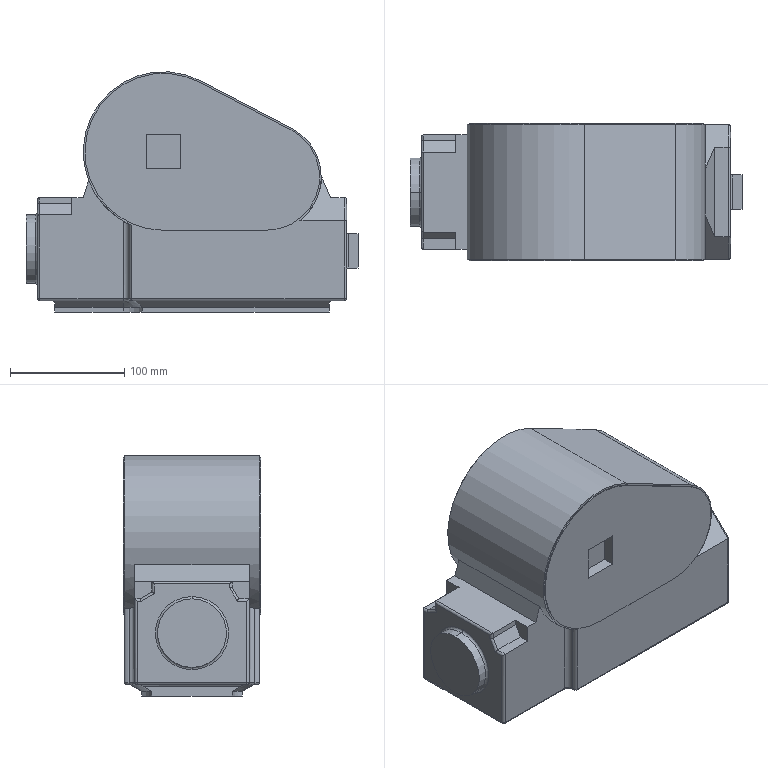Part | SolidWorks | features ICE 7, Chamfer 4, MirrorPattern 2, Extrusion 1, Fillet 1 | 1 solid | 114 faces | box 290 x 120 x 210 mm | volume 5097544 mm3 | plane 55 | cylinder 45 | torus 8 | sphere 4 | cone 2 | commonest cylinder face diameters 4 x30 10 x4 137 x3 40 x2 60 x2 93 x2